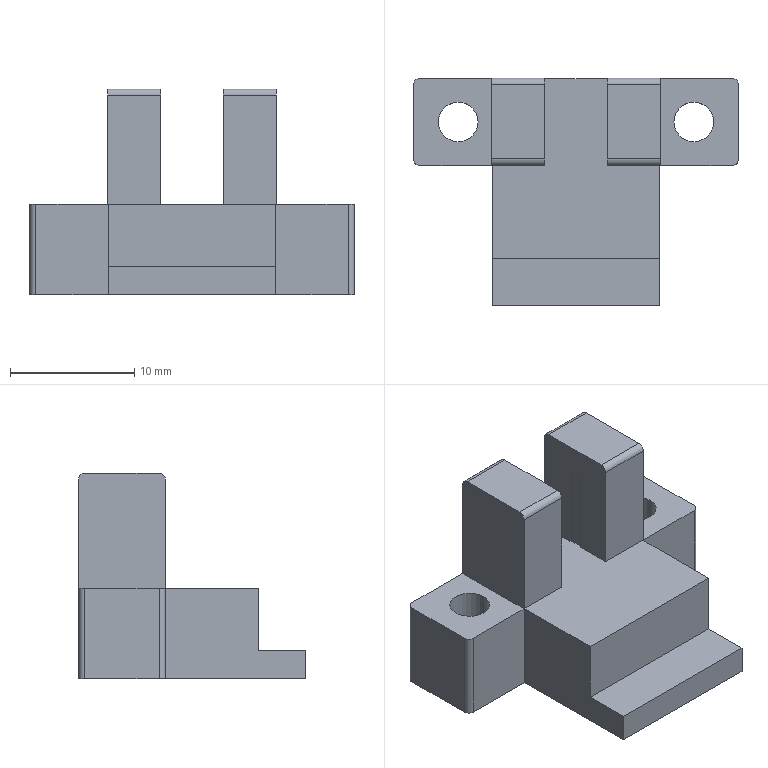Part | SolidWorks | features ICE 5, Fillet 2, Extrusion 1, MirrorPattern 1 | 1 solid | 40 faces | box 26.2 x 18.3 x 16.6 mm | volume 2634 mm3 | plane 28 | cylinder 12 | commonest cylinder face diameters 1 x8 3.2 x4
STEP:
#1=CARTESIAN_POINT('',(7.9,5.65,0.));
#2=VERTEX_POINT('',#1);
#3=CARTESIAN_POINT('',(11.1,5.65,0.));
#4=VERTEX_POINT('',#3);
#5=CARTESIAN_POINT('',(9.5,5.65,0.));
#6=DIRECTION('',(0.,0.,1.));
#7=DIRECTION('',(1.,0.,0.));
#8=AXIS2_PLACEMENT_3D('',#5,#6,#7);
#9=CIRCLE('',#8,1.6);
#10=EDGE_CURVE('',#2,#4,#9,.T.);
#11=ORIENTED_EDGE('',*,*,#10,.F.);
#12=CARTESIAN_POINT('',(7.9,5.65,7.3));
#13=VERTEX_POINT('',#12);
#14=CARTESIAN_POINT('',(7.9,5.65,-0.000025));
#15=DIRECTION('',(0.,0.,1.));
#16=VECTOR('',#15,1000.);
#17=LINE('',#14,#16);
#18=EDGE_CURVE('',#2,#13,#17,.T.);
#19=ORIENTED_EDGE('',*,*,#18,.T.);
#20=CARTESIAN_POINT('',(11.1,5.65,7.3));
#21=VERTEX_POINT('',#20);
#22=CARTESIAN_POINT('',(9.5,5.65,7.3));
#23=DIRECTION('',(0.,0.,1.));
#24=DIRECTION('',(-1.,0.,0.));
#25=AXIS2_PLACEMENT_3D('',#22,#23,#24);
#26=CIRCLE('',#25,1.6);
#27=EDGE_CURVE('',#13,#21,#26,.T.);
#28=ORIENTED_EDGE('',*,*,#27,.T.);
#29=CARTESIAN_POINT('',(11.1,5.65,-0.000025));
#30=DIRECTION('',(0.,0.,1.));
#31=VECTOR('',#30,1000.);
#32=LINE('',#29,#31);
#33=EDGE_CURVE('',#4,#21,#32,.T.);
#34=ORIENTED_EDGE('',*,*,#33,.F.);
#35=EDGE_LOOP('',(#11,#19,#28,#34));
#36=FACE_OUTER_BOUND('',#35,.T.);
#37=CARTESIAN_POINT('',(9.5,5.65,-0.000025));
#38=DIRECTION('',(0.,0.,1.));
#39=DIRECTION('',(1.,0.,0.));
#40=AXIS2_PLACEMENT_3D('',#37,#38,#39);
#41=CYLINDRICAL_SURFACE('',#40,1.6);
#42=ADVANCED_FACE('',(#36),#41,.F.);
#43=CARTESIAN_POINT('',(-11.1,5.65,0.));
#44=VERTEX_POINT('',#43);
#45=CARTESIAN_POINT('',(-7.9,5.65,0.));
#46=VERTEX_POINT('',#45);
#47=CARTESIAN_POINT('',(-9.5,5.65,0.));
#48=DIRECTION('',(0.,0.,1.));
#49=DIRECTION('',(1.,0.,0.));
#50=AXIS2_PLACEMENT_3D('',#47,#48,#49);
#51=CIRCLE('',#50,1.6);
#52=EDGE_CURVE('',#44,#46,#51,.T.);
#53=ORIENTED_EDGE('',*,*,#52,.F.);
#54=CARTESIAN_POINT('',(-11.1,5.65,7.3));
#55=VERTEX_POINT('',#54);
#56=CARTESIAN_POINT('',(-11.1,5.65,-0.000025));
#57=DIRECTION('',(0.,0.,1.));
#58=VECTOR('',#57,1000.);
#59=LINE('',#56,#58);
#60=EDGE_CURVE('',#44,#55,#59,.T.);
#61=ORIENTED_EDGE('',*,*,#60,.T.);
#62=CARTESIAN_POINT('',(-7.9,5.65,7.3));
#63=VERTEX_POINT('',#62);
#64=CARTESIAN_POINT('',(-9.5,5.65,7.3));
#65=DIRECTION('',(0.,0.,1.));
#66=DIRECTION('',(1.,0.,0.));
#67=AXIS2_PLACEMENT_3D('',#64,#65,#66);
#68=CIRCLE('',#67,1.6);
#69=EDGE_CURVE('',#55,#63,#68,.T.);
#70=ORIENTED_EDGE('',*,*,#69,.T.);
#71=CARTESIAN_POINT('',(-7.9,5.65,-0.000025));
#72=DIRECTION('',(0.,0.,1.));
#73=VECTOR('',#72,1000.);
#74=LINE('',#71,#73);
#75=EDGE_CURVE('',#46,#63,#74,.T.);
#76=ORIENTED_EDGE('',*,*,#75,.F.);
#77=EDGE_LOOP('',(#53,#61,#70,#76));
#78=FACE_OUTER_BOUND('',#77,.T.);
#79=CARTESIAN_POINT('',(-9.5,5.65,-0.000025));
#80=DIRECTION('',(0.,0.,1.));
#81=DIRECTION('',(1.,0.,0.));
#82=AXIS2_PLACEMENT_3D('',#79,#80,#81);
#83=CYLINDRICAL_SURFACE('',#82,1.6);
#84=ADVANCED_FACE('',(#78),#83,.F.);
#85=CARTESIAN_POINT('',(2.5,2.15,16.1));
#86=VERTEX_POINT('',#85);
#87=CARTESIAN_POINT('',(2.5,2.15,7.3));
#88=VERTEX_POINT('',#87);
#89=CARTESIAN_POINT('',(2.5,2.15,16.6));
#90=DIRECTION('',(0.,0.,-1.));
#91=VECTOR('',#90,1000.);
#92=LINE('',#89,#91);
#93=EDGE_CURVE('',#86,#88,#92,.T.);
#94=ORIENTED_EDGE('',*,*,#93,.F.);
#95=CARTESIAN_POINT('',(2.5,2.65,16.6));
#96=VERTEX_POINT('',#95);
#97=CARTESIAN_POINT('',(2.5,2.65,16.1));
#98=DIRECTION('',(-1.,0.,0.));
#99=DIRECTION('',(0.,1.,0.));
#100=AXIS2_PLACEMENT_3D('',#97,#98,#99);
#101=CIRCLE('',#100,0.5);
#102=EDGE_CURVE('',#86,#96,#101,.T.);
#103=ORIENTED_EDGE('',*,*,#102,.T.);
#104=CARTESIAN_POINT('',(2.5,8.65,16.6));
#105=VERTEX_POINT('',#104);
#106=CARTESIAN_POINT('',(2.5,9.15,16.6));
#107=DIRECTION('',(0.,-1.,0.));
#108=VECTOR('',#107,1000.);
#109=LINE('',#106,#108);
#110=EDGE_CURVE('',#105,#96,#109,.T.);
#111=ORIENTED_EDGE('',*,*,#110,.F.);
#112=CARTESIAN_POINT('',(2.5,9.15,16.1));
#113=VERTEX_POINT('',#112);
#114=CARTESIAN_POINT('',(2.5,8.65,16.1));
#115=DIRECTION('',(-1.,0.,0.));
#116=DIRECTION('',(0.,1.,0.));
#117=AXIS2_PLACEMENT_3D('',#114,#115,#116);
#118=CIRCLE('',#117,0.5);
#119=EDGE_CURVE('',#105,#113,#118,.T.);
#120=ORIENTED_EDGE('',*,*,#119,.T.);
#121=CARTESIAN_POINT('',(2.5,9.15,7.3));
#122=VERTEX_POINT('',#121);
#123=CARTESIAN_POINT('',(2.5,9.15,16.6));
#124=DIRECTION('',(0.,0.,-1.));
#125=VECTOR('',#124,1000.);
#126=LINE('',#123,#125);
#127=EDGE_CURVE('',#113,#122,#126,.T.);
#128=ORIENTED_EDGE('',*,*,#127,.T.);
#129=CARTESIAN_POINT('',(2.5,6.094,7.3));
#130=VERTEX_POINT('',#129);
#131=CARTESIAN_POINT('',(2.5,9.15,7.3));
#132=DIRECTION('',(0.,-1.,0.));
#133=VECTOR('',#132,1000.);
#134=LINE('',#131,#133);
#135=EDGE_CURVE('',#122,#130,#134,.T.);
#136=ORIENTED_EDGE('',*,*,#135,.T.);
#137=CARTESIAN_POINT('',(2.5,6.094,14.22));
#138=VERTEX_POINT('',#137);
#139=CARTESIAN_POINT('',(2.5,6.094,14.22));
#140=DIRECTION('',(0.,0.,1.));
#141=VECTOR('',#140,1000.);
#142=LINE('',#139,#141);
#143=EDGE_CURVE('',#130,#138,#142,.T.);
#144=ORIENTED_EDGE('',*,*,#143,.T.);
#145=CARTESIAN_POINT('',(2.5,5.036,14.22));
#146=VERTEX_POINT('',#145);
#147=CARTESIAN_POINT('',(2.5,6.094,14.22));
#148=DIRECTION('',(0.,-1.,0.));
#149=VECTOR('',#148,1000.);
#150=LINE('',#147,#149);
#151=EDGE_CURVE('',#138,#146,#150,.T.);
#152=ORIENTED_EDGE('',*,*,#151,.T.);
#153=CARTESIAN_POINT('',(2.5,5.036,7.3));
#154=VERTEX_POINT('',#153);
#155=CARTESIAN_POINT('',(2.5,5.036,14.22));
#156=DIRECTION('',(0.,0.,-1.));
#157=VECTOR('',#156,1000.);
#158=LINE('',#155,#157);
#159=EDGE_CURVE('',#146,#154,#158,.T.);
#160=ORIENTED_EDGE('',*,*,#159,.T.);
#161=CARTESIAN_POINT('',(2.5,9.15,7.3));
#162=DIRECTION('',(0.,-1.,0.));
#163=VECTOR('',#162,1000.);
#164=LINE('',#161,#163);
#165=EDGE_CURVE('',#154,#88,#164,.T.);
#166=ORIENTED_EDGE('',*,*,#165,.T.);
#167=EDGE_LOOP('',(#94,#103,#111,#120,#128,#136,#144,#152,#160,#166));
#168=FACE_OUTER_BOUND('',#167,.T.);
#169=CARTESIAN_POINT('',(2.5,9.15,16.6));
#170=DIRECTION('',(1.,0.,0.));
#171=DIRECTION('',(0.,1.,0.));
#172=AXIS2_PLACEMENT_3D('',#169,#170,#171);
#173=PLANE('',#172);
#174=ADVANCED_FACE('',(#168),#173,.F.);
#175=CARTESIAN_POINT('',(6.75,-5.35,7.3));
#176=VERTEX_POINT('',#175);
#177=CARTESIAN_POINT('',(-6.75,-5.35,7.3));
#178=VERTEX_POINT('',#177);
#179=CARTESIAN_POINT('',(-6.75,-5.35,7.3));
#180=DIRECTION('',(-1.,0.,0.));
#181=VECTOR('',#180,1000.);
#182=LINE('',#179,#181);
#183=EDGE_CURVE('',#176,#178,#182,.T.);
#184=ORIENTED_EDGE('',*,*,#183,.F.);
#185=CARTESIAN_POINT('',(6.75,2.15,7.3));
#186=VERTEX_POINT('',#185);
#187=CARTESIAN_POINT('',(6.75,2.15,7.3));
#188=DIRECTION('',(0.,-1.,0.));
#189=VECTOR('',#188,1000.);
#190=LINE('',#187,#189);
#191=EDGE_CURVE('',#186,#176,#190,.T.);
#192=ORIENTED_EDGE('',*,*,#191,.F.);
#193=CARTESIAN_POINT('',(6.8,2.15,7.3));
#194=DIRECTION('',(1.,0.,0.));
#195=VECTOR('',#194,1000.);
#196=LINE('',#193,#195);
#197=EDGE_CURVE('',#88,#186,#196,.T.);
#198=ORIENTED_EDGE('',*,*,#197,.F.);
#199=ORIENTED_EDGE('',*,*,#165,.F.);
#200=CARTESIAN_POINT('',(2.6,5.036,7.3));
#201=VERTEX_POINT('',#200);
#202=CARTESIAN_POINT('',(2.6,5.036,7.3));
#203=DIRECTION('',(-1.,0.,0.));
#204=VECTOR('',#203,1000.);
#205=LINE('',#202,#204);
#206=EDGE_CURVE('',#201,#154,#205,.T.);
#207=ORIENTED_EDGE('',*,*,#206,.F.);
#208=CARTESIAN_POINT('',(2.6,6.094,7.3));
#209=VERTEX_POINT('',#208);
#210=CARTESIAN_POINT('',(2.6,6.094,7.3));
#211=DIRECTION('',(0.,1.,0.));
#212=VECTOR('',#211,1000.);
#213=LINE('',#210,#212);
#214=EDGE_CURVE('',#201,#209,#213,.T.);
#215=ORIENTED_EDGE('',*,*,#214,.T.);
#216=CARTESIAN_POINT('',(2.6,6.094,7.3));
#217=DIRECTION('',(-1.,0.,0.));
#218=VECTOR('',#217,1000.);
#219=LINE('',#216,#218);
#220=EDGE_CURVE('',#209,#130,#219,.T.);
#221=ORIENTED_EDGE('',*,*,#220,.T.);
#222=ORIENTED_EDGE('',*,*,#135,.F.);
#223=CARTESIAN_POINT('',(-2.5,9.15,7.3));
#224=VERTEX_POINT('',#223);
#225=CARTESIAN_POINT('',(-13.1,9.15,7.3));
#226=DIRECTION('',(-1.,0.,0.));
#227=VECTOR('',#226,1000.);
#228=LINE('',#225,#227);
#229=EDGE_CURVE('',#122,#224,#228,.T.);
#230=ORIENTED_EDGE('',*,*,#229,.T.);
#231=CARTESIAN_POINT('',(-2.5,6.094,7.3));
#232=VERTEX_POINT('',#231);
#233=CARTESIAN_POINT('',(-2.5,9.15,7.3));
#234=DIRECTION('',(0.,1.,0.));
#235=VECTOR('',#234,1000.);
#236=LINE('',#233,#235);
#237=EDGE_CURVE('',#232,#224,#236,.T.);
#238=ORIENTED_EDGE('',*,*,#237,.F.);
#239=CARTESIAN_POINT('',(-2.6,6.094,7.3));
#240=VERTEX_POINT('',#239);
#241=CARTESIAN_POINT('',(-2.6,6.094,7.3));
#242=DIRECTION('',(1.,0.,0.));
#243=VECTOR('',#242,1000.);
#244=LINE('',#241,#243);
#245=EDGE_CURVE('',#240,#232,#244,.T.);
#246=ORIENTED_EDGE('',*,*,#245,.F.);
#247=CARTESIAN_POINT('',(-2.6,5.036,7.3));
#248=VERTEX_POINT('',#247);
#249=CARTESIAN_POINT('',(-2.6,6.094,7.3));
#250=DIRECTION('',(0.,1.,0.));
#251=VECTOR('',#250,1000.);
#252=LINE('',#249,#251);
#253=EDGE_CURVE('',#248,#240,#252,.T.);
#254=ORIENTED_EDGE('',*,*,#253,.F.);
#255=CARTESIAN_POINT('',(-2.5,5.036,7.3));
#256=VERTEX_POINT('',#255);
#257=CARTESIAN_POINT('',(-2.6,5.036,7.3));
#258=DIRECTION('',(1.,0.,0.));
#259=VECTOR('',#258,1000.);
#260=LINE('',#257,#259);
#261=EDGE_CURVE('',#248,#256,#260,.T.);
#262=ORIENTED_EDGE('',*,*,#261,.T.);
#263=CARTESIAN_POINT('',(-2.5,2.15,7.3));
#264=VERTEX_POINT('',#263);
#265=CARTESIAN_POINT('',(-2.5,9.15,7.3));
#266=DIRECTION('',(0.,1.,0.));
#267=VECTOR('',#266,1000.);
#268=LINE('',#265,#267);
#269=EDGE_CURVE('',#264,#256,#268,.T.);
#270=ORIENTED_EDGE('',*,*,#269,.F.);
#271=CARTESIAN_POINT('',(-6.75,2.15,7.3));
#272=VERTEX_POINT('',#271);
#273=CARTESIAN_POINT('',(-6.8,2.15,7.3));
#274=DIRECTION('',(1.,0.,0.));
#275=VECTOR('',#274,1000.);
#276=LINE('',#273,#275);
#277=EDGE_CURVE('',#272,#264,#276,.T.);
#278=ORIENTED_EDGE('',*,*,#277,.F.);
#279=CARTESIAN_POINT('',(-6.75,2.15,7.3));
#280=DIRECTION('',(0.,1.,0.));
#281=VECTOR('',#280,1000.);
#282=LINE('',#279,#281);
#283=EDGE_CURVE('',#178,#272,#282,.T.);
#284=ORIENTED_EDGE('',*,*,#283,.F.);
#285=EDGE_LOOP('',(#184,#192,#198,#199,#207,#215,#221,#222,#230,#238,#246,#254,#262,#270,#278,#284));
#286=FACE_OUTER_BOUND('',#285,.T.);
#287=CARTESIAN_POINT('',(13.1,-9.15,7.3));
#288=DIRECTION('',(0.,0.,1.));
#289=DIRECTION('',(1.,0.,0.));
#290=AXIS2_PLACEMENT_3D('',#287,#288,#289);
#291=PLANE('',#290);
#292=ADVANCED_FACE('',(#286),#291,.T.);
#293=CARTESIAN_POINT('',(9.5,5.65,7.3));
#294=DIRECTION('',(0.,0.,1.));
#295=DIRECTION('',(-1.,0.,0.));
#296=AXIS2_PLACEMENT_3D('',#293,#294,#295);
#297=CIRCLE('',#296,1.6);
#298=EDGE_CURVE('',#21,#13,#297,.T.);
#299=ORIENTED_EDGE('',*,*,#298,.F.);
#300=ORIENTED_EDGE('',*,*,#27,.F.);
#301=EDGE_LOOP('',(#299,#300));
#302=FACE_BOUND('',#301,.T.);
#303=CARTESIAN_POINT('',(12.6,2.15,7.3));
#304=VERTEX_POINT('',#303);
#305=CARTESIAN_POINT('',(6.8,2.15,7.3));
#306=VERTEX_POINT('',#305);
#307=CARTESIAN_POINT('',(13.1,2.15,7.3));
#308=DIRECTION('',(-1.,0.,0.));
#309=VECTOR('',#308,1000.);
#310=LINE('',#307,#309);
#311=EDGE_CURVE('',#304,#306,#310,.T.);
#312=ORIENTED_EDGE('',*,*,#311,.F.);
#313=CARTESIAN_POINT('',(13.1,2.65,7.3));
#314=VERTEX_POINT('',#313);
#315=CARTESIAN_POINT('',(12.6,2.65,7.3));
#316=DIRECTION('',(0.,0.,1.));
#317=DIRECTION('',(1.,0.,0.));
#318=AXIS2_PLACEMENT_3D('',#315,#316,#317);
#319=CIRCLE('',#318,0.5);
#320=EDGE_CURVE('',#304,#314,#319,.T.);
#321=ORIENTED_EDGE('',*,*,#320,.T.);
#322=CARTESIAN_POINT('',(13.1,8.65,7.3));
#323=VERTEX_POINT('',#322);
#324=CARTESIAN_POINT('',(13.1,9.15,7.3));
#325=DIRECTION('',(0.,1.,0.));
#326=VECTOR('',#325,1000.);
#327=LINE('',#324,#326);
#328=EDGE_CURVE('',#314,#323,#327,.T.);
#329=ORIENTED_EDGE('',*,*,#328,.T.);
#330=CARTESIAN_POINT('',(12.6,9.15,7.3));
#331=VERTEX_POINT('',#330);
#332=CARTESIAN_POINT('',(12.6,8.65,7.3));
#333=DIRECTION('',(0.,0.,1.));
#334=DIRECTION('',(1.,0.,0.));
#335=AXIS2_PLACEMENT_3D('',#332,#333,#334);
#336=CIRCLE('',#335,0.5);
#337=EDGE_CURVE('',#323,#331,#336,.T.);
#338=ORIENTED_EDGE('',*,*,#337,.T.);
#339=CARTESIAN_POINT('',(6.8,9.15,7.3));
#340=VERTEX_POINT('',#339);
#341=CARTESIAN_POINT('',(-13.1,9.15,7.3));
#342=DIRECTION('',(-1.,0.,0.));
#343=VECTOR('',#342,1000.);
#344=LINE('',#341,#343);
#345=EDGE_CURVE('',#331,#340,#344,.T.);
#346=ORIENTED_EDGE('',*,*,#345,.T.);
#347=CARTESIAN_POINT('',(6.8,9.15,7.3));
#348=DIRECTION('',(0.,1.,0.));
#349=VECTOR('',#348,1000.);
#350=LINE('',#347,#349);
#351=EDGE_CURVE('',#306,#340,#350,.T.);
#352=ORIENTED_EDGE('',*,*,#351,.F.);
#353=EDGE_LOOP('',(#312,#321,#329,#338,#346,#352));
#354=FACE_OUTER_BOUND('',#353,.T.);
#355=CARTESIAN_POINT('',(13.1,-9.15,7.3));
#356=DIRECTION('',(0.,0.,1.));
#357=DIRECTION('',(1.,0.,0.));
#358=AXIS2_PLACEMENT_3D('',#355,#356,#357);
#359=PLANE('',#358);
#360=ADVANCED_FACE('',(#302,#354),#359,.T.);
#361=CARTESIAN_POINT('',(-9.5,5.65,7.3));
#362=DIRECTION('',(0.,0.,1.));
#363=DIRECTION('',(1.,0.,0.));
#364=AXIS2_PLACEMENT_3D('',#361,#362,#363);
#365=CIRCLE('',#364,1.6);
#366=EDGE_CURVE('',#63,#55,#365,.T.);
#367=ORIENTED_EDGE('',*,*,#366,.F.);
#368=ORIENTED_EDGE('',*,*,#69,.F.);
#369=EDGE_LOOP('',(#367,#368));
#370=FACE_BOUND('',#369,.T.);
#371=CARTESIAN_POINT('',(-13.1,8.65,7.3));
#372=VERTEX_POINT('',#371);
#373=CARTESIAN_POINT('',(-13.1,2.65,7.3));
#374=VERTEX_POINT('',#373);
#375=CARTESIAN_POINT('',(-13.1,9.15,7.3));
#376=DIRECTION('',(0.,-1.,0.));
#377=VECTOR('',#376,1000.);
#378=LINE('',#375,#377);
#379=EDGE_CURVE('',#372,#374,#378,.T.);
#380=ORIENTED_EDGE('',*,*,#379,.T.);
#381=CARTESIAN_POINT('',(-12.6,2.15,7.3));
#382=VERTEX_POINT('',#381);
#383=CARTESIAN_POINT('',(-12.6,2.65,7.3));
#384=DIRECTION('',(0.,0.,1.));
#385=DIRECTION('',(1.,0.,0.));
#386=AXIS2_PLACEMENT_3D('',#383,#384,#385);
#387=CIRCLE('',#386,0.5);
#388=EDGE_CURVE('',#374,#382,#387,.T.);
#389=ORIENTED_EDGE('',*,*,#388,.T.);
#390=CARTESIAN_POINT('',(-6.8,2.15,7.3));
#391=VERTEX_POINT('',#390);
#392=CARTESIAN_POINT('',(-13.1,2.15,7.3));
#393=DIRECTION('',(-1.,0.,0.));
#394=VECTOR('',#393,1000.);
#395=LINE('',#392,#394);
#396=EDGE_CURVE('',#391,#382,#395,.T.);
#397=ORIENTED_EDGE('',*,*,#396,.F.);
#398=CARTESIAN_POINT('',(-6.8,9.15,7.3));
#399=VERTEX_POINT('',#398);
#400=CARTESIAN_POINT('',(-6.8,9.15,7.3));
#401=DIRECTION('',(0.,-1.,0.));
#402=VECTOR('',#401,1000.);
#403=LINE('',#400,#402);
#404=EDGE_CURVE('',#399,#391,#403,.T.);
#405=ORIENTED_EDGE('',*,*,#404,.F.);
#406=CARTESIAN_POINT('',(-12.6,9.15,7.3));
#407=VERTEX_POINT('',#406);
#408=CARTESIAN_POINT('',(-13.1,9.15,7.3));
#409=DIRECTION('',(-1.,0.,0.));
#410=VECTOR('',#409,1000.);
#411=LINE('',#408,#410);
#412=EDGE_CURVE('',#399,#407,#411,.T.);
#413=ORIENTED_EDGE('',*,*,#412,.T.);
#414=CARTESIAN_POINT('',(-12.6,8.65,7.3));
#415=DIRECTION('',(0.,0.,1.));
#416=DIRECTION('',(1.,0.,0.));
#417=AXIS2_PLACEMENT_3D('',#414,#415,#416);
#418=CIRCLE('',#417,0.5);
#419=EDGE_CURVE('',#407,#372,#418,.T.);
#420=ORIENTED_EDGE('',*,*,#419,.T.);
#421=EDGE_LOOP('',(#380,#389,#397,#405,#413,#420));
#422=FACE_OUTER_BOUND('',#421,.T.);
#423=CARTESIAN_POINT('',(13.1,-9.15,7.3));
#424=DIRECTION('',(0.,0.,1.));
#425=DIRECTION('',(1.,0.,0.));
#426=AXIS2_PLACEMENT_3D('',#423,#424,#425);
#427=PLANE('',#426);
#428=ADVANCED_FACE('',(#370,#422),#427,.T.);
#429=ORIENTED_EDGE('',*,*,#328,.F.);
#430=CARTESIAN_POINT('',(13.1,2.65,0.));
#431=VERTEX_POINT('',#430);
#432=CARTESIAN_POINT('',(13.1,2.65,7.3));
#433=DIRECTION('',(0.,0.,-1.));
#434=VECTOR('',#433,1000.);
#435=LINE('',#432,#434);
#436=EDGE_CURVE('',#314,#431,#435,.T.);
#437=ORIENTED_EDGE('',*,*,#436,.T.);
#438=CARTESIAN_POINT('',(13.1,8.65,0.));
#439=VERTEX_POINT('',#438);
#440=CARTESIAN_POINT('',(13.1,9.15,0.));
#441=DIRECTION('',(0.,1.,0.));
#442=VECTOR('',#441,1000.);
#443=LINE('',#440,#442);
#444=EDGE_CURVE('',#431,#439,#443,.T.);
#445=ORIENTED_EDGE('',*,*,#444,.T.);
#446=CARTESIAN_POINT('',(13.1,8.65,7.3));
#447=DIRECTION('',(0.,0.,1.));
#448=VECTOR('',#447,1000.);
#449=LINE('',#446,#448);
#450=EDGE_CURVE('',#439,#323,#449,.T.);
#451=ORIENTED_EDGE('',*,*,#450,.T.);
#452=EDGE_LOOP('',(#429,#437,#445,#451));
#453=FACE_OUTER_BOUND('',#452,.T.);
#454=CARTESIAN_POINT('',(13.1,9.15,7.3));
#455=DIRECTION('',(-1.,0.,0.));
#456=DIRECTION('',(0.,0.,1.));
#457=AXIS2_PLACEMENT_3D('',#454,#455,#456);
#458=PLANE('',#457);
#459=ADVANCED_FACE('',(#453),#458,.F.);
#460=ORIENTED_EDGE('',*,*,#127,.F.);
#461=CARTESIAN_POINT('',(6.8,9.15,16.1));
#462=VERTEX_POINT('',#461);
#463=CARTESIAN_POINT('',(6.8,9.15,16.1));
#464=DIRECTION('',(1.,0.,0.));
#465=VECTOR('',#464,1000.);
#466=LINE('',#463,#465);
#467=EDGE_CURVE('',#113,#462,#466,.T.);
#468=ORIENTED_EDGE('',*,*,#467,.T.);
#469=CARTESIAN_POINT('',(6.8,9.15,16.6));
#470=DIRECTION('',(0.,0.,-1.));
#471=VECTOR('',#470,1000.);
#472=LINE('',#469,#471);
#473=EDGE_CURVE('',#462,#340,#472,.T.);
#474=ORIENTED_EDGE('',*,*,#473,.T.);
#475=ORIENTED_EDGE('',*,*,#345,.F.);
#476=CARTESIAN_POINT('',(12.6,9.15,0.));
#477=VERTEX_POINT('',#476);
#478=CARTESIAN_POINT('',(12.6,9.15,7.3));
#479=DIRECTION('',(0.,0.,-1.));
#480=VECTOR('',#479,1000.);
#481=LINE('',#478,#480);
#482=EDGE_CURVE('',#331,#477,#481,.T.);
#483=ORIENTED_EDGE('',*,*,#482,.T.);
#484=CARTESIAN_POINT('',(-12.6,9.15,0.));
#485=VERTEX_POINT('',#484);
#486=CARTESIAN_POINT('',(-13.1,9.15,0.));
#487=DIRECTION('',(-1.,0.,0.));
#488=VECTOR('',#487,1000.);
#489=LINE('',#486,#488);
#490=EDGE_CURVE('',#477,#485,#489,.T.);
#491=ORIENTED_EDGE('',*,*,#490,.T.);
#492=CARTESIAN_POINT('',(-12.6,9.15,7.3));
#493=DIRECTION('',(0.,0.,1.));
#494=VECTOR('',#493,1000.);
#495=LINE('',#492,#494);
#496=EDGE_CURVE('',#485,#407,#495,.T.);
#497=ORIENTED_EDGE('',*,*,#496,.T.);
#498=ORIENTED_EDGE('',*,*,#412,.F.);
#499=CARTESIAN_POINT('',(-6.8,9.15,16.1));
#500=VERTEX_POINT('',#499);
#501=CARTESIAN_POINT('',(-6.8,9.15,16.6));
#502=DIRECTION('',(0.,0.,-1.));
#503=VECTOR('',#502,1000.);
#504=LINE('',#501,#503);
#505=EDGE_CURVE('',#500,#399,#504,.T.);
#506=ORIENTED_EDGE('',*,*,#505,.F.);
#507=CARTESIAN_POINT('',(-2.5,9.15,16.1));
#508=VERTEX_POINT('',#507);
#509=CARTESIAN_POINT('',(-2.5,9.15,16.1));
#510=DIRECTION('',(1.,0.,0.));
#511=VECTOR('',#510,1000.);
#512=LINE('',#509,#511);
#513=EDGE_CURVE('',#500,#508,#512,.T.);
#514=ORIENTED_EDGE('',*,*,#513,.T.);
#515=CARTESIAN_POINT('',(-2.5,9.15,16.6));
#516=DIRECTION('',(0.,0.,-1.));
#517=VECTOR('',#516,1000.);
#518=LINE('',#515,#517);
#519=EDGE_CURVE('',#508,#224,#518,.T.);
#520=ORIENTED_EDGE('',*,*,#519,.T.);
#521=ORIENTED_EDGE('',*,*,#229,.F.);
#522=EDGE_LOOP('',(#460,#468,#474,#475,#483,#491,#497,#498,#506,#514,#520,#521));
#523=FACE_OUTER_BOUND('',#522,.T.);
#524=CARTESIAN_POINT('',(-13.1,9.15,7.3));
#525=DIRECTION('',(0.,-1.,0.));
#526=DIRECTION('',(0.,0.,-1.));
#527=AXIS2_PLACEMENT_3D('',#524,#525,#526);
#528=PLANE('',#527);
#529=ADVANCED_FACE('',(#523),#528,.F.);
#530=CARTESIAN_POINT('',(-13.1,8.65,0.));
#531=VERTEX_POINT('',#530);
#532=CARTESIAN_POINT('',(-13.1,2.65,0.));
#533=VERTEX_POINT('',#532);
#534=CARTESIAN_POINT('',(-13.1,9.15,0.));
#535=DIRECTION('',(0.,-1.,0.));
#536=VECTOR('',#535,1000.);
#537=LINE('',#534,#536);
#538=EDGE_CURVE('',#531,#533,#537,.T.);
#539=ORIENTED_EDGE('',*,*,#538,.T.);
#540=CARTESIAN_POINT('',(-13.1,2.65,7.3));
#541=DIRECTION('',(0.,0.,1.));
#542=VECTOR('',#541,1000.);
#543=LINE('',#540,#542);
#544=EDGE_CURVE('',#533,#374,#543,.T.);
#545=ORIENTED_EDGE('',*,*,#544,.T.);
#546=ORIENTED_EDGE('',*,*,#379,.F.);
#547=CARTESIAN_POINT('',(-13.1,8.65,7.3));
#548=DIRECTION('',(0.,0.,-1.));
#549=VECTOR('',#548,1000.);
#550=LINE('',#547,#549);
#551=EDGE_CURVE('',#372,#531,#550,.T.);
#552=ORIENTED_EDGE('',*,*,#551,.T.);
#553=EDGE_LOOP('',(#539,#545,#546,#552));
#554=FACE_OUTER_BOUND('',#553,.T.);
#555=CARTESIAN_POINT('',(-13.1,9.15,7.3));
#556=DIRECTION('',(1.,0.,0.));
#557=DIRECTION('',(0.,1.,0.));
#558=AXIS2_PLACEMENT_3D('',#555,#556,#557);
#559=PLANE('',#558);
#560=ADVANCED_FACE('',(#554),#559,.F.);
#561=CARTESIAN_POINT('',(6.75,-9.15,0.));
#562=VERTEX_POINT('',#561);
#563=CARTESIAN_POINT('',(6.75,-9.15,2.3));
#564=VERTEX_POINT('',#563);
#565=CARTESIAN_POINT('',(6.75,-9.15,0.));
#566=DIRECTION('',(0.,0.,1.));
#567=VECTOR('',#566,1000.);
#568=LINE('',#565,#567);
#569=EDGE_CURVE('',#562,#564,#568,.T.);
#570=ORIENTED_EDGE('',*,*,#569,.T.);
#571=CARTESIAN_POINT('',(-6.75,-9.15,2.3));
#572=VERTEX_POINT('',#571);
#573=CARTESIAN_POINT('',(-6.75,-9.15,2.3));
#574=DIRECTION('',(1.,0.,0.));
#575=VECTOR('',#574,1000.);
#576=LINE('',#573,#575);
#577=EDGE_CURVE('',#572,#564,#576,.T.);
#578=ORIENTED_EDGE('',*,*,#577,.F.);
#579=CARTESIAN_POINT('',(-6.75,-9.15,0.));
#580=VERTEX_POINT('',#579);
#581=CARTESIAN_POINT('',(-6.75,-9.15,0.));
#582=DIRECTION('',(0.,0.,1.));
#583=VECTOR('',#582,1000.);
#584=LINE('',#581,#583);
#585=EDGE_CURVE('',#580,#572,#584,.T.);
#586=ORIENTED_EDGE('',*,*,#585,.F.);
#587=CARTESIAN_POINT('',(-13.1,-9.15,0.));
#588=DIRECTION('',(1.,0.,0.));
#589=VECTOR('',#588,1000.);
#590=LINE('',#587,#589);
#591=EDGE_CURVE('',#580,#562,#590,.T.);
#592=ORIENTED_EDGE('',*,*,#591,.T.);
#593=EDGE_LOOP('',(#570,#578,#586,#592));
#594=FACE_OUTER_BOUND('',#593,.T.);
#595=CARTESIAN_POINT('',(-13.1,-9.15,7.3));
#596=DIRECTION('',(0.,1.,0.));
#597=DIRECTION('',(0.,0.,1.));
#598=AXIS2_PLACEMENT_3D('',#595,#596,#597);
#599=PLANE('',#598);
#600=ADVANCED_FACE('',(#594),#599,.F.);
#601=CARTESIAN_POINT('',(9.5,5.65,0.));
#602=DIRECTION('',(0.,0.,1.));
#603=DIRECTION('',(1.,0.,0.));
#604=AXIS2_PLACEMENT_3D('',#601,#602,#603);
#605=CIRCLE('',#604,1.6);
#606=EDGE_CURVE('',#4,#2,#605,.T.);
#607=ORIENTED_EDGE('',*,*,#606,.T.);
#608=ORIENTED_EDGE('',*,*,#10,.T.);
#609=EDGE_LOOP('',(#607,#608));
#610=FACE_BOUND('',#609,.T.);
#611=CARTESIAN_POINT('',(-9.5,5.65,0.));
#612=DIRECTION('',(0.,0.,1.));
#613=DIRECTION('',(1.,0.,0.));
#614=AXIS2_PLACEMENT_3D('',#611,#612,#613);
#615=CIRCLE('',#614,1.6);
#616=EDGE_CURVE('',#46,#44,#615,.T.);
#617=ORIENTED_EDGE('',*,*,#616,.T.);
#618=ORIENTED_EDGE('',*,*,#52,.T.);
#619=EDGE_LOOP('',(#617,#618));
#620=FACE_BOUND('',#619,.T.);
#621=ORIENTED_EDGE('',*,*,#444,.F.);
#622=CARTESIAN_POINT('',(12.6,2.15,0.));
#623=VERTEX_POINT('',#622);
#624=CARTESIAN_POINT('',(12.6,2.65,0.));
#625=DIRECTION('',(0.,0.,-1.));
#626=DIRECTION('',(1.,0.,0.));
#627=AXIS2_PLACEMENT_3D('',#624,#625,#626);
#628=CIRCLE('',#627,0.5);
#629=EDGE_CURVE('',#431,#623,#628,.T.);
#630=ORIENTED_EDGE('',*,*,#629,.T.);
#631=CARTESIAN_POINT('',(6.75,2.15,0.));
#632=VERTEX_POINT('',#631);
#633=CARTESIAN_POINT('',(13.1,2.15,0.));
#634=DIRECTION('',(-1.,0.,0.));
#635=VECTOR('',#634,1000.);
#636=LINE('',#633,#635);
#637=EDGE_CURVE('',#623,#632,#636,.T.);
#638=ORIENTED_EDGE('',*,*,#637,.T.);
#639=CARTESIAN_POINT('',(6.75,2.15,0.));
#640=DIRECTION('',(0.,-1.,0.));
#641=VECTOR('',#640,1000.);
#642=LINE('',#639,#641);
#643=EDGE_CURVE('',#632,#562,#642,.T.);
#644=ORIENTED_EDGE('',*,*,#643,.T.);
#645=ORIENTED_EDGE('',*,*,#591,.F.);
#646=CARTESIAN_POINT('',(-6.75,2.15,0.));
#647=VERTEX_POINT('',#646);
#648=CARTESIAN_POINT('',(-6.75,2.15,0.));
#649=DIRECTION('',(0.,1.,0.));
#650=VECTOR('',#649,1000.);
#651=LINE('',#648,#650);
#652=EDGE_CURVE('',#580,#647,#651,.T.);
#653=ORIENTED_EDGE('',*,*,#652,.T.);
#654=CARTESIAN_POINT('',(-12.6,2.15,0.));
#655=VERTEX_POINT('',#654);
#656=CARTESIAN_POINT('',(-13.1,2.15,0.));
#657=DIRECTION('',(-1.,0.,0.));
#658=VECTOR('',#657,1000.);
#659=LINE('',#656,#658);
#660=EDGE_CURVE('',#647,#655,#659,.T.);
#661=ORIENTED_EDGE('',*,*,#660,.T.);
#662=CARTESIAN_POINT('',(-12.6,2.65,0.));
#663=DIRECTION('',(0.,0.,-1.));
#664=DIRECTION('',(1.,0.,0.));
#665=AXIS2_PLACEMENT_3D('',#662,#663,#664);
#666=CIRCLE('',#665,0.5);
#667=EDGE_CURVE('',#655,#533,#666,.T.);
#668=ORIENTED_EDGE('',*,*,#667,.T.);
#669=ORIENTED_EDGE('',*,*,#538,.F.);
#670=CARTESIAN_POINT('',(-12.6,8.65,0.));
#671=DIRECTION('',(0.,0.,-1.));
#672=DIRECTION('',(1.,0.,0.));
#673=AXIS2_PLACEMENT_3D('',#670,#671,#672);
#674=CIRCLE('',#673,0.5);
#675=EDGE_CURVE('',#531,#485,#674,.T.);
#676=ORIENTED_EDGE('',*,*,#675,.T.);
#677=ORIENTED_EDGE('',*,*,#490,.F.);
#678=CARTESIAN_POINT('',(12.6,8.65,0.));
#679=DIRECTION('',(0.,0.,-1.));
#680=DIRECTION('',(1.,0.,0.));
#681=AXIS2_PLACEMENT_3D('',#678,#679,#680);
#682=CIRCLE('',#681,0.5);
#683=EDGE_CURVE('',#477,#439,#682,.T.);
#684=ORIENTED_EDGE('',*,*,#683,.T.);
#685=EDGE_LOOP('',(#621,#630,#638,#644,#645,#653,#661,#668,#669,#676,#677,#684));
#686=FACE_OUTER_BOUND('',#685,.T.);
#687=CARTESIAN_POINT('',(13.1,-9.15,0.));
#688=DIRECTION('',(0.,0.,1.));
#689=DIRECTION('',(1.,0.,0.));
#690=AXIS2_PLACEMENT_3D('',#687,#688,#689);
#691=PLANE('',#690);
#692=ADVANCED_FACE('',(#610,#620,#686),#691,.F.);
#693=CARTESIAN_POINT('',(-2.5,2.15,16.1));
#694=VERTEX_POINT('',#693);
#695=CARTESIAN_POINT('',(-2.5,2.15,16.6));
#696=DIRECTION('',(0.,0.,-1.));
#697=VECTOR('',#696,1000.);
#698=LINE('',#695,#697);
#699=EDGE_CURVE('',#694,#264,#698,.T.);
#700=ORIENTED_EDGE('',*,*,#699,.F.);
#701=CARTESIAN_POINT('',(-6.8,2.15,16.1));
#702=VERTEX_POINT('',#701);
#703=CARTESIAN_POINT('',(-6.8,2.15,16.1));
#704=DIRECTION('',(-1.,0.,0.));
#705=VECTOR('',#704,1000.);
#706=LINE('',#703,#705);
#707=EDGE_CURVE('',#694,#702,#706,.T.);
#708=ORIENTED_EDGE('',*,*,#707,.T.);
#709=CARTESIAN_POINT('',(-6.8,2.15,16.6));
#710=DIRECTION('',(0.,0.,-1.));
#711=VECTOR('',#710,1000.);
#712=LINE('',#709,#711);
#713=EDGE_CURVE('',#702,#391,#712,.T.);
#714=ORIENTED_EDGE('',*,*,#713,.T.);
#715=ORIENTED_EDGE('',*,*,#396,.T.);
#716=CARTESIAN_POINT('',(-12.6,2.15,0.));
#717=DIRECTION('',(0.,0.,-1.));
#718=VECTOR('',#717,1000.);
#719=LINE('',#716,#718);
#720=EDGE_CURVE('',#382,#655,#719,.T.);
#721=ORIENTED_EDGE('',*,*,#720,.T.);
#722=ORIENTED_EDGE('',*,*,#660,.F.);
#723=CARTESIAN_POINT('',(-6.75,2.15,0.));
#724=DIRECTION('',(0.,0.,1.));
#725=VECTOR('',#724,1000.);
#726=LINE('',#723,#725);
#727=EDGE_CURVE('',#647,#272,#726,.T.);
#728=ORIENTED_EDGE('',*,*,#727,.T.);
#729=ORIENTED_EDGE('',*,*,#277,.T.);
#730=EDGE_LOOP('',(#700,#708,#714,#715,#721,#722,#728,#729));
#731=FACE_OUTER_BOUND('',#730,.T.);
#732=CARTESIAN_POINT('',(-13.1,2.15,0.));
#733=DIRECTION('',(0.,1.,0.));
#734=DIRECTION('',(-1.,0.,0.));
#735=AXIS2_PLACEMENT_3D('',#732,#733,#734);
#736=PLANE('',#735);
#737=ADVANCED_FACE('',(#731),#736,.F.);
#738=CARTESIAN_POINT('',(-6.75,-5.35,2.3));
#739=VERTEX_POINT('',#738);
#740=CARTESIAN_POINT('',(-6.75,-9.15,2.3));
#741=DIRECTION('',(0.,-1.,0.));
#742=VECTOR('',#741,1000.);
#743=LINE('',#740,#742);
#744=EDGE_CURVE('',#739,#572,#743,.T.);
#745=ORIENTED_EDGE('',*,*,#744,.F.);
#746=CARTESIAN_POINT('',(-6.75,-5.35,2.3));
#747=DIRECTION('',(0.,0.,1.));
#748=VECTOR('',#747,1000.);
#749=LINE('',#746,#748);
#750=EDGE_CURVE('',#739,#178,#749,.T.);
#751=ORIENTED_EDGE('',*,*,#750,.T.);
#752=ORIENTED_EDGE('',*,*,#283,.T.);
#753=ORIENTED_EDGE('',*,*,#727,.F.);
#754=ORIENTED_EDGE('',*,*,#652,.F.);
#755=ORIENTED_EDGE('',*,*,#585,.T.);
#756=EDGE_LOOP('',(#745,#751,#752,#753,#754,#755));
#757=FACE_OUTER_BOUND('',#756,.T.);
#758=CARTESIAN_POINT('',(-6.75,2.15,0.));
#759=DIRECTION('',(1.,0.,0.));
#760=DIRECTION('',(0.,1.,0.));
#761=AXIS2_PLACEMENT_3D('',#758,#759,#760);
#762=PLANE('',#761);
#763=ADVANCED_FACE('',(#757),#762,.F.);
#764=CARTESIAN_POINT('',(6.8,2.15,16.1));
#765=VERTEX_POINT('',#764);
#766=CARTESIAN_POINT('',(6.8,2.15,16.6));
#767=DIRECTION('',(0.,0.,-1.));
#768=VECTOR('',#767,1000.);
#769=LINE('',#766,#768);
#770=EDGE_CURVE('',#765,#306,#769,.T.);
#771=ORIENTED_EDGE('',*,*,#770,.F.);
#772=CARTESIAN_POINT('',(2.5,2.15,16.1));
#773=DIRECTION('',(-1.,0.,0.));
#774=VECTOR('',#773,1000.);
#775=LINE('',#772,#774);
#776=EDGE_CURVE('',#765,#86,#775,.T.);
#777=ORIENTED_EDGE('',*,*,#776,.T.);
#778=ORIENTED_EDGE('',*,*,#93,.T.);
#779=ORIENTED_EDGE('',*,*,#197,.T.);
#780=CARTESIAN_POINT('',(6.75,2.15,0.));
#781=DIRECTION('',(0.,0.,1.));
#782=VECTOR('',#781,1000.);
#783=LINE('',#780,#782);
#784=EDGE_CURVE('',#632,#186,#783,.T.);
#785=ORIENTED_EDGE('',*,*,#784,.F.);
#786=ORIENTED_EDGE('',*,*,#637,.F.);
#787=CARTESIAN_POINT('',(12.6,2.15,0.));
#788=DIRECTION('',(0.,0.,1.));
#789=VECTOR('',#788,1000.);
#790=LINE('',#787,#789);
#791=EDGE_CURVE('',#623,#304,#790,.T.);
#792=ORIENTED_EDGE('',*,*,#791,.T.);
#793=ORIENTED_EDGE('',*,*,#311,.T.);
#794=EDGE_LOOP('',(#771,#777,#778,#779,#785,#786,#792,#793));
#795=FACE_OUTER_BOUND('',#794,.T.);
#796=CARTESIAN_POINT('',(13.1,2.15,0.));
#797=DIRECTION('',(0.,1.,0.));
#798=DIRECTION('',(-1.,0.,0.));
#799=AXIS2_PLACEMENT_3D('',#796,#797,#798);
#800=PLANE('',#799);
#801=ADVANCED_FACE('',(#795),#800,.F.);
#802=ORIENTED_EDGE('',*,*,#191,.T.);
#803=CARTESIAN_POINT('',(6.75,-5.35,2.3));
#804=VERTEX_POINT('',#803);
#805=CARTESIAN_POINT('',(6.75,-5.35,2.3));
#806=DIRECTION('',(0.,0.,1.));
#807=VECTOR('',#806,1000.);
#808=LINE('',#805,#807);
#809=EDGE_CURVE('',#804,#176,#808,.T.);
#810=ORIENTED_EDGE('',*,*,#809,.F.);
#811=CARTESIAN_POINT('',(6.75,-9.15,2.3));
#812=DIRECTION('',(0.,1.,0.));
#813=VECTOR('',#812,1000.);
#814=LINE('',#811,#813);
#815=EDGE_CURVE('',#564,#804,#814,.T.);
#816=ORIENTED_EDGE('',*,*,#815,.F.);
#817=ORIENTED_EDGE('',*,*,#569,.F.);
#818=ORIENTED_EDGE('',*,*,#643,.F.);
#819=ORIENTED_EDGE('',*,*,#784,.T.);
#820=EDGE_LOOP('',(#802,#810,#816,#817,#818,#819));
#821=FACE_OUTER_BOUND('',#820,.T.);
#822=CARTESIAN_POINT('',(6.75,2.15,0.));
#823=DIRECTION('',(-1.,0.,0.));
#824=DIRECTION('',(0.,-1.,0.));
#825=AXIS2_PLACEMENT_3D('',#822,#823,#824);
#826=PLANE('',#825);
#827=ADVANCED_FACE('',(#821),#826,.F.);
#828=CARTESIAN_POINT('',(-6.8,8.65,16.6));
#829=VERTEX_POINT('',#828);
#830=CARTESIAN_POINT('',(-6.8,2.65,16.6));
#831=VERTEX_POINT('',#830);
#832=CARTESIAN_POINT('',(-6.8,9.15,16.6));
#833=DIRECTION('',(0.,-1.,0.));
#834=VECTOR('',#833,1000.);
#835=LINE('',#832,#834);
#836=EDGE_CURVE('',#829,#831,#835,.T.);
#837=ORIENTED_EDGE('',*,*,#836,.F.);
#838=CARTESIAN_POINT('',(-6.8,8.65,16.1));
#839=DIRECTION('',(-1.,0.,0.));
#840=DIRECTION('',(0.,0.,-1.));
#841=AXIS2_PLACEMENT_3D('',#838,#839,#840);
#842=CIRCLE('',#841,0.5);
#843=EDGE_CURVE('',#829,#500,#842,.T.);
#844=ORIENTED_EDGE('',*,*,#843,.T.);
#845=ORIENTED_EDGE('',*,*,#505,.T.);
#846=ORIENTED_EDGE('',*,*,#404,.T.);
#847=ORIENTED_EDGE('',*,*,#713,.F.);
#848=CARTESIAN_POINT('',(-6.8,2.65,16.1));
#849=DIRECTION('',(-1.,0.,0.));
#850=DIRECTION('',(0.,0.,-1.));
#851=AXIS2_PLACEMENT_3D('',#848,#849,#850);
#852=CIRCLE('',#851,0.5);
#853=EDGE_CURVE('',#702,#831,#852,.T.);
#854=ORIENTED_EDGE('',*,*,#853,.T.);
#855=EDGE_LOOP('',(#837,#844,#845,#846,#847,#854));
#856=FACE_OUTER_BOUND('',#855,.T.);
#857=CARTESIAN_POINT('',(-6.8,9.15,16.6));
#858=DIRECTION('',(1.,0.,0.));
#859=DIRECTION('',(0.,0.,-1.));
#860=AXIS2_PLACEMENT_3D('',#857,#858,#859);
#861=PLANE('',#860);
#862=ADVANCED_FACE('',(#856),#861,.F.);
#863=ORIENTED_EDGE('',*,*,#519,.F.);
#864=CARTESIAN_POINT('',(-2.5,8.65,16.6));
#865=VERTEX_POINT('',#864);
#866=CARTESIAN_POINT('',(-2.5,8.65,16.1));
#867=DIRECTION('',(1.,0.,0.));
#868=DIRECTION('',(0.,-1.,0.));
#869=AXIS2_PLACEMENT_3D('',#866,#867,#868);
#870=CIRCLE('',#869,0.5);
#871=EDGE_CURVE('',#508,#865,#870,.T.);
#872=ORIENTED_EDGE('',*,*,#871,.T.);
#873=CARTESIAN_POINT('',(-2.5,2.65,16.6));
#874=VERTEX_POINT('',#873);
#875=CARTESIAN_POINT('',(-2.5,9.15,16.6));
#876=DIRECTION('',(0.,1.,0.));
#877=VECTOR('',#876,1000.);
#878=LINE('',#875,#877);
#879=EDGE_CURVE('',#874,#865,#878,.T.);
#880=ORIENTED_EDGE('',*,*,#879,.F.);
#881=CARTESIAN_POINT('',(-2.5,2.65,16.1));
#882=DIRECTION('',(1.,0.,0.));
#883=DIRECTION('',(0.,-1.,0.));
#884=AXIS2_PLACEMENT_3D('',#881,#882,#883);
#885=CIRCLE('',#884,0.5);
#886=EDGE_CURVE('',#874,#694,#885,.T.);
#887=ORIENTED_EDGE('',*,*,#886,.T.);
#888=ORIENTED_EDGE('',*,*,#699,.T.);
#889=ORIENTED_EDGE('',*,*,#269,.T.);
#890=CARTESIAN_POINT('',(-2.5,5.036,14.22));
#891=VERTEX_POINT('',#890);
#892=CARTESIAN_POINT('',(-2.5,5.036,14.22));
#893=DIRECTION('',(0.,0.,-1.));
#894=VECTOR('',#893,1000.);
#895=LINE('',#892,#894);
#896=EDGE_CURVE('',#891,#256,#895,.T.);
#897=ORIENTED_EDGE('',*,*,#896,.F.);
#898=CARTESIAN_POINT('',(-2.5,6.094,14.22));
#899=VERTEX_POINT('',#898);
#900=CARTESIAN_POINT('',(-2.5,6.094,14.22));
#901=DIRECTION('',(0.,-1.,0.));
#902=VECTOR('',#901,1000.);
#903=LINE('',#900,#902);
#904=EDGE_CURVE('',#899,#891,#903,.T.);
#905=ORIENTED_EDGE('',*,*,#904,.F.);
#906=CARTESIAN_POINT('',(-2.5,6.094,14.22));
#907=DIRECTION('',(0.,0.,1.));
#908=VECTOR('',#907,1000.);
#909=LINE('',#906,#908);
#910=EDGE_CURVE('',#232,#899,#909,.T.);
#911=ORIENTED_EDGE('',*,*,#910,.F.);
#912=ORIENTED_EDGE('',*,*,#237,.T.);
#913=EDGE_LOOP('',(#863,#872,#880,#887,#888,#889,#897,#905,#911,#912));
#914=FACE_OUTER_BOUND('',#913,.T.);
#915=CARTESIAN_POINT('',(-2.5,9.15,16.6));
#916=DIRECTION('',(-1.,0.,0.));
#917=DIRECTION('',(0.,-1.,0.));
#918=AXIS2_PLACEMENT_3D('',#915,#916,#917);
#919=PLANE('',#918);
#920=ADVANCED_FACE('',(#914),#919,.F.);
#921=ORIENTED_EDGE('',*,*,#879,.T.);
#922=CARTESIAN_POINT('',(-6.8,8.65,16.6));
#923=DIRECTION('',(-1.,0.,0.));
#924=VECTOR('',#923,1000.);
#925=LINE('',#922,#924);
#926=EDGE_CURVE('',#865,#829,#925,.T.);
#927=ORIENTED_EDGE('',*,*,#926,.T.);
#928=ORIENTED_EDGE('',*,*,#836,.T.);
#929=CARTESIAN_POINT('',(-2.5,2.65,16.6));
#930=DIRECTION('',(1.,0.,0.));
#931=VECTOR('',#930,1000.);
#932=LINE('',#929,#931);
#933=EDGE_CURVE('',#831,#874,#932,.T.);
#934=ORIENTED_EDGE('',*,*,#933,.T.);
#935=EDGE_LOOP('',(#921,#927,#928,#934));
#936=FACE_OUTER_BOUND('',#935,.T.);
#937=CARTESIAN_POINT('',(-6.8,2.15,16.6));
#938=DIRECTION('',(0.,0.,1.));
#939=DIRECTION('',(1.,0.,0.));
#940=AXIS2_PLACEMENT_3D('',#937,#938,#939);
#941=PLANE('',#940);
#942=ADVANCED_FACE('',(#936),#941,.T.);
#943=CARTESIAN_POINT('',(6.8,2.65,16.6));
#944=VERTEX_POINT('',#943);
#945=CARTESIAN_POINT('',(6.8,8.65,16.6));
#946=VERTEX_POINT('',#945);
#947=CARTESIAN_POINT('',(6.8,9.15,16.6));
#948=DIRECTION('',(0.,1.,0.));
#949=VECTOR('',#948,1000.);
#950=LINE('',#947,#949);
#951=EDGE_CURVE('',#944,#946,#950,.T.);
#952=ORIENTED_EDGE('',*,*,#951,.F.);
#953=CARTESIAN_POINT('',(6.8,2.65,16.1));
#954=DIRECTION('',(1.,0.,0.));
#955=DIRECTION('',(0.,0.,1.));
#956=AXIS2_PLACEMENT_3D('',#953,#954,#955);
#957=CIRCLE('',#956,0.5);
#958=EDGE_CURVE('',#944,#765,#957,.T.);
#959=ORIENTED_EDGE('',*,*,#958,.T.);
#960=ORIENTED_EDGE('',*,*,#770,.T.);
#961=ORIENTED_EDGE('',*,*,#351,.T.);
#962=ORIENTED_EDGE('',*,*,#473,.F.);
#963=CARTESIAN_POINT('',(6.8,8.65,16.1));
#964=DIRECTION('',(1.,0.,0.));
#965=DIRECTION('',(0.,0.,1.));
#966=AXIS2_PLACEMENT_3D('',#963,#964,#965);
#967=CIRCLE('',#966,0.5);
#968=EDGE_CURVE('',#462,#946,#967,.T.);
#969=ORIENTED_EDGE('',*,*,#968,.T.);
#970=EDGE_LOOP('',(#952,#959,#960,#961,#962,#969));
#971=FACE_OUTER_BOUND('',#970,.T.);
#972=CARTESIAN_POINT('',(6.8,9.15,16.6));
#973=DIRECTION('',(-1.,0.,0.));
#974=DIRECTION('',(0.,0.,1.));
#975=AXIS2_PLACEMENT_3D('',#972,#973,#974);
#976=PLANE('',#975);
#977=ADVANCED_FACE('',(#971),#976,.F.);
#978=ORIENTED_EDGE('',*,*,#110,.T.);
#979=CARTESIAN_POINT('',(6.8,2.65,16.6));
#980=DIRECTION('',(1.,0.,0.));
#981=VECTOR('',#980,1000.);
#982=LINE('',#979,#981);
#983=EDGE_CURVE('',#96,#944,#982,.T.);
#984=ORIENTED_EDGE('',*,*,#983,.T.);
#985=ORIENTED_EDGE('',*,*,#951,.T.);
#986=CARTESIAN_POINT('',(2.5,8.65,16.6));
#987=DIRECTION('',(-1.,0.,0.));
#988=VECTOR('',#987,1000.);
#989=LINE('',#986,#988);
#990=EDGE_CURVE('',#946,#105,#989,.T.);
#991=ORIENTED_EDGE('',*,*,#990,.T.);
#992=EDGE_LOOP('',(#978,#984,#985,#991));
#993=FACE_OUTER_BOUND('',#992,.T.);
#994=CARTESIAN_POINT('',(2.5,9.15,16.6));
#995=DIRECTION('',(0.,0.,1.));
#996=DIRECTION('',(1.,0.,0.));
#997=AXIS2_PLACEMENT_3D('',#994,#995,#996);
#998=PLANE('',#997);
#999=ADVANCED_FACE('',(#993),#998,.T.);
#1000=ORIENTED_EDGE('',*,*,#183,.T.);
#1001=ORIENTED_EDGE('',*,*,#750,.F.);
#1002=CARTESIAN_POINT('',(-6.75,-5.35,2.3));
#1003=DIRECTION('',(-1.,0.,0.));
#1004=VECTOR('',#1003,1000.);
#1005=LINE('',#1002,#1004);
#1006=EDGE_CURVE('',#804,#739,#1005,.T.);
#1007=ORIENTED_EDGE('',*,*,#1006,.F.);
#1008=ORIENTED_EDGE('',*,*,#809,.T.);
#1009=EDGE_LOOP('',(#1000,#1001,#1007,#1008));
#1010=FACE_OUTER_BOUND('',#1009,.T.);
#1011=CARTESIAN_POINT('',(-6.75,-5.35,2.3));
#1012=DIRECTION('',(0.,1.,0.));
#1013=DIRECTION('',(0.,0.,1.));
#1014=AXIS2_PLACEMENT_3D('',#1011,#1012,#1013);
#1015=PLANE('',#1014);
#1016=ADVANCED_FACE('',(#1010),#1015,.F.);
#1017=ORIENTED_EDGE('',*,*,#744,.T.);
#1018=ORIENTED_EDGE('',*,*,#577,.T.);
#1019=ORIENTED_EDGE('',*,*,#815,.T.);
#1020=ORIENTED_EDGE('',*,*,#1006,.T.);
#1021=EDGE_LOOP('',(#1017,#1018,#1019,#1020));
#1022=FACE_OUTER_BOUND('',#1021,.T.);
#1023=CARTESIAN_POINT('',(-6.75,-5.35,2.3));
#1024=DIRECTION('',(0.,0.,-1.));
#1025=DIRECTION('',(-1.,0.,0.));
#1026=AXIS2_PLACEMENT_3D('',#1023,#1024,#1025);
#1027=PLANE('',#1026);
#1028=ADVANCED_FACE('',(#1022),#1027,.F.);
#1029=ORIENTED_EDGE('',*,*,#60,.F.);
#1030=ORIENTED_EDGE('',*,*,#616,.F.);
#1031=ORIENTED_EDGE('',*,*,#75,.T.);
#1032=ORIENTED_EDGE('',*,*,#366,.T.);
#1033=EDGE_LOOP('',(#1029,#1030,#1031,#1032));
#1034=FACE_OUTER_BOUND('',#1033,.T.);
#1035=CARTESIAN_POINT('',(-9.5,5.65,-0.000025));
#1036=DIRECTION('',(0.,0.,1.));
#1037=DIRECTION('',(1.,0.,0.));
#1038=AXIS2_PLACEMENT_3D('',#1035,#1036,#1037);
#1039=CYLINDRICAL_SURFACE('',#1038,1.6);
#1040=ADVANCED_FACE('',(#1034),#1039,.F.);
#1041=ORIENTED_EDGE('',*,*,#18,.F.);
#1042=ORIENTED_EDGE('',*,*,#606,.F.);
#1043=ORIENTED_EDGE('',*,*,#33,.T.);
#1044=ORIENTED_EDGE('',*,*,#298,.T.);
#1045=EDGE_LOOP('',(#1041,#1042,#1043,#1044));
#1046=FACE_OUTER_BOUND('',#1045,.T.);
#1047=CARTESIAN_POINT('',(9.5,5.65,-0.000025));
#1048=DIRECTION('',(0.,0.,1.));
#1049=DIRECTION('',(1.,0.,0.));
#1050=AXIS2_PLACEMENT_3D('',#1047,#1048,#1049);
#1051=CYLINDRICAL_SURFACE('',#1050,1.6);
#1052=ADVANCED_FACE('',(#1046),#1051,.F.);
#1053=ORIENTED_EDGE('',*,*,#904,.T.);
#1054=CARTESIAN_POINT('',(-2.6,5.036,14.22));
#1055=VERTEX_POINT('',#1054);
#1056=CARTESIAN_POINT('',(-2.6,5.036,14.22));
#1057=DIRECTION('',(1.,0.,0.));
#1058=VECTOR('',#1057,1000.);
#1059=LINE('',#1056,#1058);
#1060=EDGE_CURVE('',#1055,#891,#1059,.T.);
#1061=ORIENTED_EDGE('',*,*,#1060,.F.);
#1062=CARTESIAN_POINT('',(-2.6,6.094,14.22));
#1063=VERTEX_POINT('',#1062);
#1064=CARTESIAN_POINT('',(-2.6,6.094,14.22));
#1065=DIRECTION('',(0.,-1.,0.));
#1066=VECTOR('',#1065,1000.);
#1067=LINE('',#1064,#1066);
#1068=EDGE_CURVE('',#1063,#1055,#1067,.T.);
#1069=ORIENTED_EDGE('',*,*,#1068,.F.);
#1070=CARTESIAN_POINT('',(-2.6,6.094,14.22));
#1071=DIRECTION('',(1.,0.,0.));
#1072=VECTOR('',#1071,1000.);
#1073=LINE('',#1070,#1072);
#1074=EDGE_CURVE('',#1063,#899,#1073,.T.);
#1075=ORIENTED_EDGE('',*,*,#1074,.T.);
#1076=EDGE_LOOP('',(#1053,#1061,#1069,#1075));
#1077=FACE_OUTER_BOUND('',#1076,.T.);
#1078=CARTESIAN_POINT('',(-2.6,6.094,14.22));
#1079=DIRECTION('',(0.,0.,1.));
#1080=DIRECTION('',(1.,0.,0.));
#1081=AXIS2_PLACEMENT_3D('',#1078,#1079,#1080);
#1082=PLANE('',#1081);
#1083=ADVANCED_FACE('',(#1077),#1082,.F.);
#1084=ORIENTED_EDGE('',*,*,#910,.T.);
#1085=ORIENTED_EDGE('',*,*,#1074,.F.);
#1086=CARTESIAN_POINT('',(-2.6,6.094,14.22));
#1087=DIRECTION('',(0.,0.,1.));
#1088=VECTOR('',#1087,1000.);
#1089=LINE('',#1086,#1088);
#1090=EDGE_CURVE('',#240,#1063,#1089,.T.);
#1091=ORIENTED_EDGE('',*,*,#1090,.F.);
#1092=ORIENTED_EDGE('',*,*,#245,.T.);
#1093=EDGE_LOOP('',(#1084,#1085,#1091,#1092));
#1094=FACE_OUTER_BOUND('',#1093,.T.);
#1095=CARTESIAN_POINT('',(-2.6,6.094,14.22));
#1096=DIRECTION('',(0.,1.,0.));
#1097=DIRECTION('',(-1.,0.,0.));
#1098=AXIS2_PLACEMENT_3D('',#1095,#1096,#1097);
#1099=PLANE('',#1098);
#1100=ADVANCED_FACE('',(#1094),#1099,.F.);
#1101=ORIENTED_EDGE('',*,*,#896,.T.);
#1102=ORIENTED_EDGE('',*,*,#261,.F.);
#1103=CARTESIAN_POINT('',(-2.6,5.036,14.22));
#1104=DIRECTION('',(0.,0.,-1.));
#1105=VECTOR('',#1104,1000.);
#1106=LINE('',#1103,#1105);
#1107=EDGE_CURVE('',#1055,#248,#1106,.T.);
#1108=ORIENTED_EDGE('',*,*,#1107,.F.);
#1109=ORIENTED_EDGE('',*,*,#1060,.T.);
#1110=EDGE_LOOP('',(#1101,#1102,#1108,#1109));
#1111=FACE_OUTER_BOUND('',#1110,.T.);
#1112=CARTESIAN_POINT('',(-2.6,5.036,14.22));
#1113=DIRECTION('',(0.,-1.,0.));
#1114=DIRECTION('',(1.,0.,0.));
#1115=AXIS2_PLACEMENT_3D('',#1112,#1113,#1114);
#1116=PLANE('',#1115);
#1117=ADVANCED_FACE('',(#1111),#1116,.F.);
#1118=ORIENTED_EDGE('',*,*,#1068,.T.);
#1119=ORIENTED_EDGE('',*,*,#1107,.T.);
#1120=ORIENTED_EDGE('',*,*,#253,.T.);
#1121=ORIENTED_EDGE('',*,*,#1090,.T.);
#1122=EDGE_LOOP('',(#1118,#1119,#1120,#1121));
#1123=FACE_OUTER_BOUND('',#1122,.T.);
#1124=CARTESIAN_POINT('',(-2.6,5.036,14.22));
#1125=DIRECTION('',(1.,0.,0.));
#1126=DIRECTION('',(0.,1.,0.));
#1127=AXIS2_PLACEMENT_3D('',#1124,#1125,#1126);
#1128=PLANE('',#1127);
#1129=ADVANCED_FACE('',(#1123),#1128,.T.);
#1130=ORIENTED_EDGE('',*,*,#629,.F.);
#1131=ORIENTED_EDGE('',*,*,#436,.F.);
#1132=ORIENTED_EDGE('',*,*,#320,.F.);
#1133=ORIENTED_EDGE('',*,*,#791,.F.);
#1134=EDGE_LOOP('',(#1130,#1131,#1132,#1133));
#1135=FACE_OUTER_BOUND('',#1134,.T.);
#1136=CARTESIAN_POINT('',(12.6,2.65,0.));
#1137=DIRECTION('',(0.,0.,1.));
#1138=DIRECTION('',(1.,0.,0.));
#1139=AXIS2_PLACEMENT_3D('',#1136,#1137,#1138);
#1140=CYLINDRICAL_SURFACE('',#1139,0.5);
#1141=ADVANCED_FACE('',(#1135),#1140,.T.);
#1142=ORIENTED_EDGE('',*,*,#337,.F.);
#1143=ORIENTED_EDGE('',*,*,#450,.F.);
#1144=ORIENTED_EDGE('',*,*,#683,.F.);
#1145=ORIENTED_EDGE('',*,*,#482,.F.);
#1146=EDGE_LOOP('',(#1142,#1143,#1144,#1145));
#1147=FACE_OUTER_BOUND('',#1146,.T.);
#1148=CARTESIAN_POINT('',(12.6,8.65,7.3));
#1149=DIRECTION('',(0.,0.,-1.));
#1150=DIRECTION('',(-1.,0.,0.));
#1151=AXIS2_PLACEMENT_3D('',#1148,#1149,#1150);
#1152=CYLINDRICAL_SURFACE('',#1151,0.5);
#1153=ADVANCED_FACE('',(#1147),#1152,.T.);
#1154=ORIENTED_EDGE('',*,*,#667,.F.);
#1155=ORIENTED_EDGE('',*,*,#720,.F.);
#1156=ORIENTED_EDGE('',*,*,#388,.F.);
#1157=ORIENTED_EDGE('',*,*,#544,.F.);
#1158=EDGE_LOOP('',(#1154,#1155,#1156,#1157));
#1159=FACE_OUTER_BOUND('',#1158,.T.);
#1160=CARTESIAN_POINT('',(-12.6,2.65,7.3));
#1161=DIRECTION('',(0.,0.,1.));
#1162=DIRECTION('',(1.,0.,0.));
#1163=AXIS2_PLACEMENT_3D('',#1160,#1161,#1162);
#1164=CYLINDRICAL_SURFACE('',#1163,0.5);
#1165=ADVANCED_FACE('',(#1159),#1164,.T.);
#1166=ORIENTED_EDGE('',*,*,#419,.F.);
#1167=ORIENTED_EDGE('',*,*,#496,.F.);
#1168=ORIENTED_EDGE('',*,*,#675,.F.);
#1169=ORIENTED_EDGE('',*,*,#551,.F.);
#1170=EDGE_LOOP('',(#1166,#1167,#1168,#1169));
#1171=FACE_OUTER_BOUND('',#1170,.T.);
#1172=CARTESIAN_POINT('',(-12.6,8.65,7.3));
#1173=DIRECTION('',(0.,0.,-1.));
#1174=DIRECTION('',(-1.,0.,0.));
#1175=AXIS2_PLACEMENT_3D('',#1172,#1173,#1174);
#1176=CYLINDRICAL_SURFACE('',#1175,0.5);
#1177=ADVANCED_FACE('',(#1171),#1176,.T.);
#1178=ORIENTED_EDGE('',*,*,#151,.F.);
#1179=CARTESIAN_POINT('',(2.6,6.094,14.22));
#1180=VERTEX_POINT('',#1179);
#1181=CARTESIAN_POINT('',(2.6,6.094,14.22));
#1182=DIRECTION('',(-1.,0.,0.));
#1183=VECTOR('',#1182,1000.);
#1184=LINE('',#1181,#1183);
#1185=EDGE_CURVE('',#1180,#138,#1184,.T.);
#1186=ORIENTED_EDGE('',*,*,#1185,.F.);
#1187=CARTESIAN_POINT('',(2.6,5.036,14.22));
#1188=VERTEX_POINT('',#1187);
#1189=CARTESIAN_POINT('',(2.6,6.094,14.22));
#1190=DIRECTION('',(0.,-1.,0.));
#1191=VECTOR('',#1190,1000.);
#1192=LINE('',#1189,#1191);
#1193=EDGE_CURVE('',#1180,#1188,#1192,.T.);
#1194=ORIENTED_EDGE('',*,*,#1193,.T.);
#1195=CARTESIAN_POINT('',(2.6,5.036,14.22));
#1196=DIRECTION('',(-1.,0.,0.));
#1197=VECTOR('',#1196,1000.);
#1198=LINE('',#1195,#1197);
#1199=EDGE_CURVE('',#1188,#146,#1198,.T.);
#1200=ORIENTED_EDGE('',*,*,#1199,.T.);
#1201=EDGE_LOOP('',(#1178,#1186,#1194,#1200));
#1202=FACE_OUTER_BOUND('',#1201,.T.);
#1203=CARTESIAN_POINT('',(2.6,6.094,14.22));
#1204=DIRECTION('',(0.,0.,-1.));
#1205=DIRECTION('',(-1.,0.,0.));
#1206=AXIS2_PLACEMENT_3D('',#1203,#1204,#1205);
#1207=PLANE('',#1206);
#1208=ADVANCED_FACE('',(#1202),#1207,.T.);
#1209=ORIENTED_EDGE('',*,*,#159,.F.);
#1210=ORIENTED_EDGE('',*,*,#1199,.F.);
#1211=CARTESIAN_POINT('',(2.6,5.036,14.22));
#1212=DIRECTION('',(0.,0.,-1.));
#1213=VECTOR('',#1212,1000.);
#1214=LINE('',#1211,#1213);
#1215=EDGE_CURVE('',#1188,#201,#1214,.T.);
#1216=ORIENTED_EDGE('',*,*,#1215,.T.);
#1217=ORIENTED_EDGE('',*,*,#206,.T.);
#1218=EDGE_LOOP('',(#1209,#1210,#1216,#1217));
#1219=FACE_OUTER_BOUND('',#1218,.T.);
#1220=CARTESIAN_POINT('',(2.6,5.036,14.22));
#1221=DIRECTION('',(0.,1.,0.));
#1222=DIRECTION('',(-1.,0.,0.));
#1223=AXIS2_PLACEMENT_3D('',#1220,#1221,#1222);
#1224=PLANE('',#1223);
#1225=ADVANCED_FACE('',(#1219),#1224,.T.);
#1226=ORIENTED_EDGE('',*,*,#143,.F.);
#1227=ORIENTED_EDGE('',*,*,#220,.F.);
#1228=CARTESIAN_POINT('',(2.6,6.094,14.22));
#1229=DIRECTION('',(0.,0.,1.));
#1230=VECTOR('',#1229,1000.);
#1231=LINE('',#1228,#1230);
#1232=EDGE_CURVE('',#209,#1180,#1231,.T.);
#1233=ORIENTED_EDGE('',*,*,#1232,.T.);
#1234=ORIENTED_EDGE('',*,*,#1185,.T.);
#1235=EDGE_LOOP('',(#1226,#1227,#1233,#1234));
#1236=FACE_OUTER_BOUND('',#1235,.T.);
#1237=CARTESIAN_POINT('',(2.6,6.094,14.22));
#1238=DIRECTION('',(0.,-1.,0.));
#1239=DIRECTION('',(1.,0.,0.));
#1240=AXIS2_PLACEMENT_3D('',#1237,#1238,#1239);
#1241=PLANE('',#1240);
#1242=ADVANCED_FACE('',(#1236),#1241,.T.);
#1243=ORIENTED_EDGE('',*,*,#1193,.F.);
#1244=ORIENTED_EDGE('',*,*,#1232,.F.);
#1245=ORIENTED_EDGE('',*,*,#214,.F.);
#1246=ORIENTED_EDGE('',*,*,#1215,.F.);
#1247=EDGE_LOOP('',(#1243,#1244,#1245,#1246));
#1248=FACE_OUTER_BOUND('',#1247,.T.);
#1249=CARTESIAN_POINT('',(2.6,0.,0.));
#1250=DIRECTION('',(-1.,0.,0.));
#1251=DIRECTION('',(0.,1.,0.));
#1252=AXIS2_PLACEMENT_3D('',#1249,#1250,#1251);
#1253=PLANE('',#1252);
#1254=ADVANCED_FACE('',(#1248),#1253,.T.);
#1255=ORIENTED_EDGE('',*,*,#102,.F.);
#1256=ORIENTED_EDGE('',*,*,#776,.F.);
#1257=ORIENTED_EDGE('',*,*,#958,.F.);
#1258=ORIENTED_EDGE('',*,*,#983,.F.);
#1259=EDGE_LOOP('',(#1255,#1256,#1257,#1258));
#1260=FACE_OUTER_BOUND('',#1259,.T.);
#1261=CARTESIAN_POINT('',(2.5,2.65,16.1));
#1262=DIRECTION('',(-1.,0.,0.));
#1263=DIRECTION('',(0.,-1.,0.));
#1264=AXIS2_PLACEMENT_3D('',#1261,#1262,#1263);
#1265=CYLINDRICAL_SURFACE('',#1264,0.5);
#1266=ADVANCED_FACE('',(#1260),#1265,.T.);
#1267=ORIENTED_EDGE('',*,*,#968,.F.);
#1268=ORIENTED_EDGE('',*,*,#467,.F.);
#1269=ORIENTED_EDGE('',*,*,#119,.F.);
#1270=ORIENTED_EDGE('',*,*,#990,.F.);
#1271=EDGE_LOOP('',(#1267,#1268,#1269,#1270));
#1272=FACE_OUTER_BOUND('',#1271,.T.);
#1273=CARTESIAN_POINT('',(2.5,8.65,16.1));
#1274=DIRECTION('',(1.,0.,0.));
#1275=DIRECTION('',(0.,0.,-1.));
#1276=AXIS2_PLACEMENT_3D('',#1273,#1274,#1275);
#1277=CYLINDRICAL_SURFACE('',#1276,0.5);
#1278=ADVANCED_FACE('',(#1272),#1277,.T.);
#1279=ORIENTED_EDGE('',*,*,#871,.F.);
#1280=ORIENTED_EDGE('',*,*,#513,.F.);
#1281=ORIENTED_EDGE('',*,*,#843,.F.);
#1282=ORIENTED_EDGE('',*,*,#926,.F.);
#1283=EDGE_LOOP('',(#1279,#1280,#1281,#1282));
#1284=FACE_OUTER_BOUND('',#1283,.T.);
#1285=CARTESIAN_POINT('',(-6.8,8.65,16.1));
#1286=DIRECTION('',(1.,0.,0.));
#1287=DIRECTION('',(0.,0.,-1.));
#1288=AXIS2_PLACEMENT_3D('',#1285,#1286,#1287);
#1289=CYLINDRICAL_SURFACE('',#1288,0.5);
#1290=ADVANCED_FACE('',(#1284),#1289,.T.);
#1291=ORIENTED_EDGE('',*,*,#853,.F.);
#1292=ORIENTED_EDGE('',*,*,#707,.F.);
#1293=ORIENTED_EDGE('',*,*,#886,.F.);
#1294=ORIENTED_EDGE('',*,*,#933,.F.);
#1295=EDGE_LOOP('',(#1291,#1292,#1293,#1294));
#1296=FACE_OUTER_BOUND('',#1295,.T.);
#1297=CARTESIAN_POINT('',(-6.8,2.65,16.1));
#1298=DIRECTION('',(-1.,0.,0.));
#1299=DIRECTION('',(0.,-1.,0.));
#1300=AXIS2_PLACEMENT_3D('',#1297,#1298,#1299);
#1301=CYLINDRICAL_SURFACE('',#1300,0.5);
#1302=ADVANCED_FACE('',(#1296),#1301,.T.);
#1303=CLOSED_SHELL('',(#42,#84,#174,#292,#360,#428,#459,#529,#560,#600,#692,#737,#763,#801,#827,#862,#920,#942,#977,#999,#1016,#1028,#1040,#1052,#1083,#1100,#1117,#1129,#1141,#1153,#1165,#1177,#1208,#1225,#1242,#1254,#1266,#1278,#1290,#1302));
#1304=MANIFOLD_SOLID_BREP('',#1303);
#1305=CARTESIAN_POINT('',(0.,0.,0.));
#1306=DIRECTION('',(0.,0.,1.));
#1307=DIRECTION('',(1.,0.,0.));
#1308=AXIS2_PLACEMENT_3D('',#1305,#1306,#1307);
#1309=(LENGTH_UNIT()NAMED_UNIT(*)SI_UNIT(.MILLI.,.METRE.));
#1310=UNCERTAINTY_MEASURE_WITH_UNIT(LENGTH_MEASURE(0.00001),#1309,'','');
#1311=(NAMED_UNIT(*)PLANE_ANGLE_UNIT()SI_UNIT($,.RADIAN.));
#1312=(NAMED_UNIT(*)SI_UNIT($,.STERADIAN.)SOLID_ANGLE_UNIT());
#1313=(GEOMETRIC_REPRESENTATION_CONTEXT(3)GLOBAL_UNCERTAINTY_ASSIGNED_CONTEXT((#1310))GLOBAL_UNIT_ASSIGNED_CONTEXT((#1309,#1311,#1312))REPRESENTATION_CONTEXT('',''));
#1314=ADVANCED_BREP_SHAPE_REPRESENTATION('',(#1304,#1308),#1313);